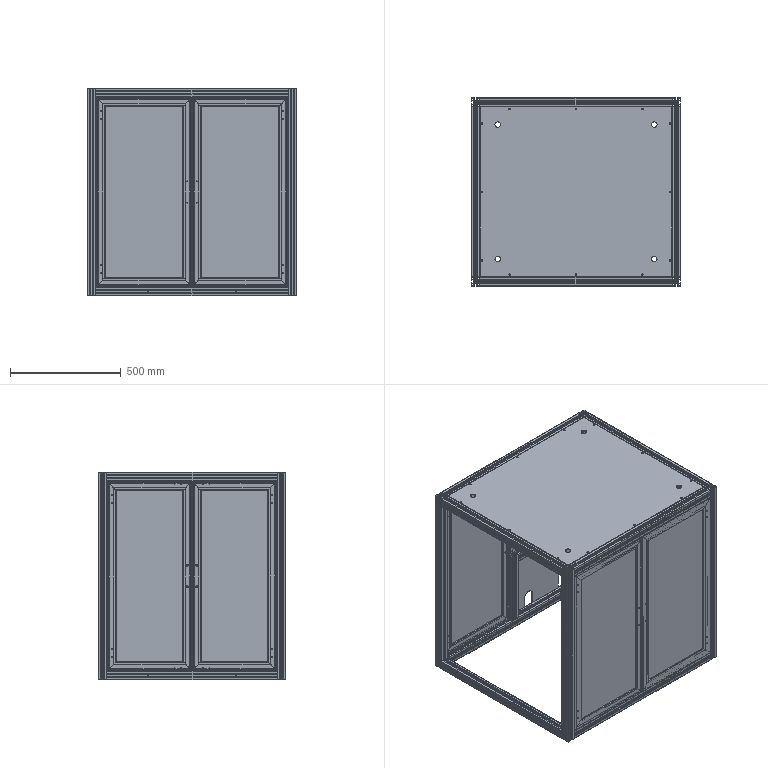Part | SolidWorks | 47 solids | 3396 faces | volume 21354940 mm3 | plane 2539 | cylinder 809 | cone 48 | commonest cylinder face diameters 13.3 x293 5 x96 12 x60 0.6 x56 7 x56 3.3 x48